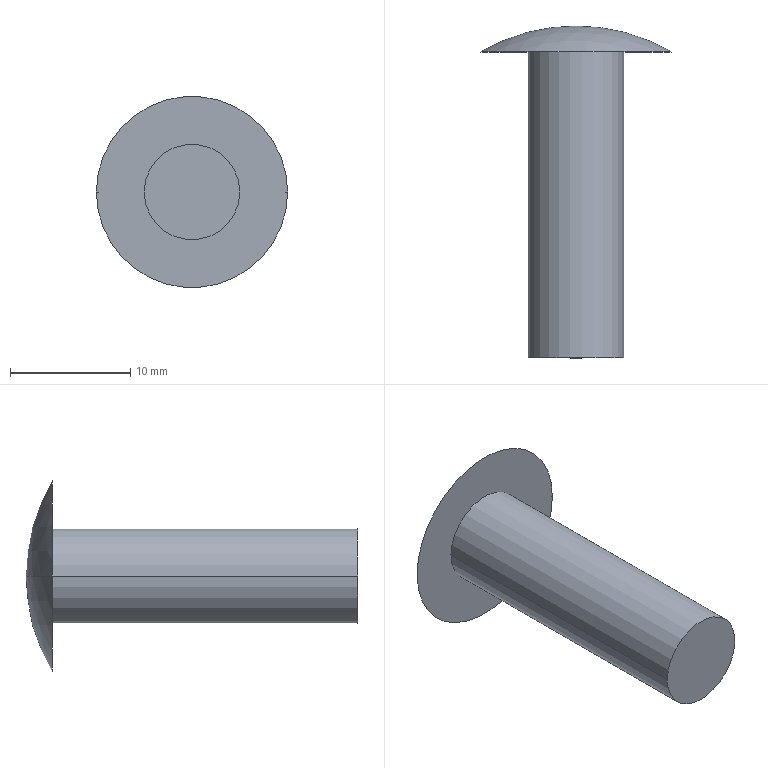Part | NX | features BREP 1 | 1 solid | 6 faces | box 15.875 x 27.559 x 15.875 mm | volume 1476 mm3 | plane 2 | sphere 2 | cylinder 2 | commonest cylinder face diameters 7.938 x2
STEP:
#1=CARTESIAN_POINT('',(-7.938,0.,0.));
#2=VERTEX_POINT('',#1);
#3=CARTESIAN_POINT('',(7.938,0.,0.));
#4=VERTEX_POINT('',#3);
#5=CARTESIAN_POINT('',(0.,0.,0.));
#6=DIRECTION('',(0.,1.,0.));
#7=DIRECTION('',(-1.,0.,0.));
#8=AXIS2_PLACEMENT_3D('',#5,#6,#7);
#9=CIRCLE('',#8,7.938);
#10=EDGE_CURVE('',#2,#4,#9,.T.);
#11=ORIENTED_EDGE('',*,*,#10,.F.);
#12=CARTESIAN_POINT('',(0.,0.,0.));
#13=DIRECTION('',(0.,-1.,0.));
#14=DIRECTION('',(-1.,0.,0.));
#15=AXIS2_PLACEMENT_3D('',#12,#13,#14);
#16=CIRCLE('',#15,7.938);
#17=EDGE_CURVE('',#2,#4,#16,.T.);
#18=ORIENTED_EDGE('',*,*,#17,.T.);
#19=EDGE_LOOP('',(#11,#18));
#20=FACE_BOUND('',#19,.T.);
#21=CARTESIAN_POINT('',(-3.969,0.,0.));
#22=VERTEX_POINT('',#21);
#23=CARTESIAN_POINT('',(3.969,0.,0.));
#24=VERTEX_POINT('',#23);
#25=CARTESIAN_POINT('',(0.,0.,0.));
#26=DIRECTION('',(0.,-1.,0.));
#27=DIRECTION('',(-1.,0.,0.));
#28=AXIS2_PLACEMENT_3D('',#25,#26,#27);
#29=CIRCLE('',#28,3.969);
#30=EDGE_CURVE('',#22,#24,#29,.T.);
#31=ORIENTED_EDGE('',*,*,#30,.F.);
#32=CARTESIAN_POINT('',(0.,0.,0.));
#33=DIRECTION('',(0.,1.,0.));
#34=DIRECTION('',(-1.,0.,0.));
#35=AXIS2_PLACEMENT_3D('',#32,#33,#34);
#36=CIRCLE('',#35,3.969);
#37=EDGE_CURVE('',#22,#24,#36,.T.);
#38=ORIENTED_EDGE('',*,*,#37,.T.);
#39=EDGE_LOOP('',(#31,#38));
#40=FACE_BOUND('',#39,.T.);
#41=CARTESIAN_POINT('',(0.,0.,0.));
#42=DIRECTION('',(0.,-1.,0.));
#43=DIRECTION('',(0.,0.,-1.));
#44=AXIS2_PLACEMENT_3D('',#41,#42,#43);
#45=PLANE('',#44);
#46=ADVANCED_FACE('',(#20,#40),#45,.T.);
#47=CARTESIAN_POINT('',(0.,-13.511,0.));
#48=DIRECTION('',(0.,0.,1.));
#49=DIRECTION('',(0.5065,0.8622,0.));
#50=AXIS2_PLACEMENT_3D('',#47,#48,#49);
#51=CIRCLE('',#50,15.67);
#52=EDGE_CURVE('',#4,#2,#51,.T.);
#53=ORIENTED_EDGE('',*,*,#52,.F.);
#54=ORIENTED_EDGE('',*,*,#17,.F.);
#55=EDGE_LOOP('',(#53,#54));
#56=FACE_BOUND('',#55,.T.);
#57=CARTESIAN_POINT('',(0.,-13.511,0.));
#58=DIRECTION('',(0.,0.,1.));
#59=DIRECTION('',(1.,0.,0.));
#60=AXIS2_PLACEMENT_3D('',#57,#58,#59);
#61=SPHERICAL_SURFACE('',#60,15.67);
#62=ADVANCED_FACE('',(#56),#61,.T.);
#63=ORIENTED_EDGE('',*,*,#10,.T.);
#64=ORIENTED_EDGE('',*,*,#52,.T.);
#65=EDGE_LOOP('',(#63,#64));
#66=FACE_BOUND('',#65,.T.);
#67=CARTESIAN_POINT('',(0.,-13.511,0.));
#68=DIRECTION('',(0.,0.,1.));
#69=DIRECTION('',(1.,0.,0.));
#70=AXIS2_PLACEMENT_3D('',#67,#68,#69);
#71=SPHERICAL_SURFACE('',#70,15.67);
#72=ADVANCED_FACE('',(#66),#71,.T.);
#73=CARTESIAN_POINT('',(-3.969,-25.4,0.));
#74=VERTEX_POINT('',#73);
#75=CARTESIAN_POINT('',(3.969,-25.4,0.));
#76=VERTEX_POINT('',#75);
#77=CARTESIAN_POINT('',(0.,-25.4,0.));
#78=DIRECTION('',(0.,1.,0.));
#79=DIRECTION('',(-1.,0.,0.));
#80=AXIS2_PLACEMENT_3D('',#77,#78,#79);
#81=CIRCLE('',#80,3.969);
#82=EDGE_CURVE('',#74,#76,#81,.T.);
#83=ORIENTED_EDGE('',*,*,#82,.T.);
#84=CARTESIAN_POINT('',(3.969,-25.4,0.));
#85=DIRECTION('',(0.,1.,0.));
#86=VECTOR('',#85,1000.);
#87=LINE('',#84,#86);
#88=EDGE_CURVE('',#76,#24,#87,.T.);
#89=ORIENTED_EDGE('',*,*,#88,.T.);
#90=ORIENTED_EDGE('',*,*,#37,.F.);
#91=CARTESIAN_POINT('',(-3.969,-25.4,0.));
#92=DIRECTION('',(0.,1.,0.));
#93=VECTOR('',#92,1000.);
#94=LINE('',#91,#93);
#95=EDGE_CURVE('',#74,#22,#94,.T.);
#96=ORIENTED_EDGE('',*,*,#95,.F.);
#97=EDGE_LOOP('',(#83,#89,#90,#96));
#98=FACE_BOUND('',#97,.T.);
#99=CARTESIAN_POINT('',(0.,3.537,0.));
#100=DIRECTION('',(0.,-1.,0.));
#101=DIRECTION('',(1.,0.,0.));
#102=AXIS2_PLACEMENT_3D('',#99,#100,#101);
#103=CYLINDRICAL_SURFACE('',#102,3.969);
#104=ADVANCED_FACE('',(#98),#103,.T.);
#105=ORIENTED_EDGE('',*,*,#30,.T.);
#106=ORIENTED_EDGE('',*,*,#88,.F.);
#107=CARTESIAN_POINT('',(0.,-25.4,0.));
#108=DIRECTION('',(0.,-1.,0.));
#109=DIRECTION('',(-1.,0.,0.));
#110=AXIS2_PLACEMENT_3D('',#107,#108,#109);
#111=CIRCLE('',#110,3.969);
#112=EDGE_CURVE('',#74,#76,#111,.T.);
#113=ORIENTED_EDGE('',*,*,#112,.F.);
#114=ORIENTED_EDGE('',*,*,#95,.T.);
#115=EDGE_LOOP('',(#105,#106,#113,#114));
#116=FACE_BOUND('',#115,.T.);
#117=CARTESIAN_POINT('',(0.,3.537,0.));
#118=DIRECTION('',(0.,-1.,0.));
#119=DIRECTION('',(1.,0.,0.));
#120=AXIS2_PLACEMENT_3D('',#117,#118,#119);
#121=CYLINDRICAL_SURFACE('',#120,3.969);
#122=ADVANCED_FACE('',(#116),#121,.T.);
#123=ORIENTED_EDGE('',*,*,#112,.T.);
#124=ORIENTED_EDGE('',*,*,#82,.F.);
#125=EDGE_LOOP('',(#123,#124));
#126=FACE_BOUND('',#125,.T.);
#127=CARTESIAN_POINT('',(0.,-25.4,0.));
#128=DIRECTION('',(0.,-1.,0.));
#129=DIRECTION('',(0.,0.,-1.));
#130=AXIS2_PLACEMENT_3D('',#127,#128,#129);
#131=PLANE('',#130);
#132=ADVANCED_FACE('',(#126),#131,.T.);
#133=CLOSED_SHELL('',(#46,#62,#72,#104,#122,#132));
#134=MANIFOLD_SOLID_BREP('',#133);
#135=(LENGTH_UNIT()NAMED_UNIT(*)SI_UNIT(.MILLI.,.METRE.));
#136=UNCERTAINTY_MEASURE_WITH_UNIT(LENGTH_MEASURE(0.00001),#135,'','');
#137=(NAMED_UNIT(*)PLANE_ANGLE_UNIT()SI_UNIT($,.RADIAN.));
#138=(NAMED_UNIT(*)SI_UNIT($,.STERADIAN.)SOLID_ANGLE_UNIT());
#139=(GEOMETRIC_REPRESENTATION_CONTEXT(3)GLOBAL_UNCERTAINTY_ASSIGNED_CONTEXT((#136))GLOBAL_UNIT_ASSIGNED_CONTEXT((#135,#137,#138))REPRESENTATION_CONTEXT('',''));
#140=ADVANCED_BREP_SHAPE_REPRESENTATION('',(#134),#139);